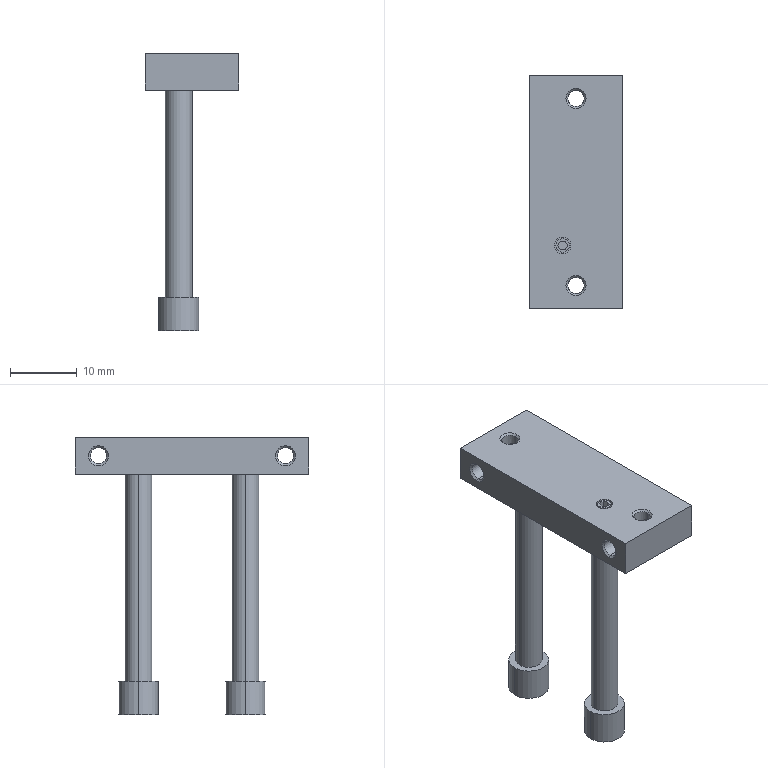Part | SolidWorks | features ICE 4, RevCut 4, RefAxis 3, Revolution 2, 3DProfileFeature 1, Extrusion 1 | 1 solid | 76 faces | box 14 x 35 x 41.5 mm | volume 3580 mm3 | cylinder 32 | plane 28 | cone 16 | commonest cylinder face diameters 2.459 x16 2.5 x4 4 x4 6 x4 2 x2 3 x2